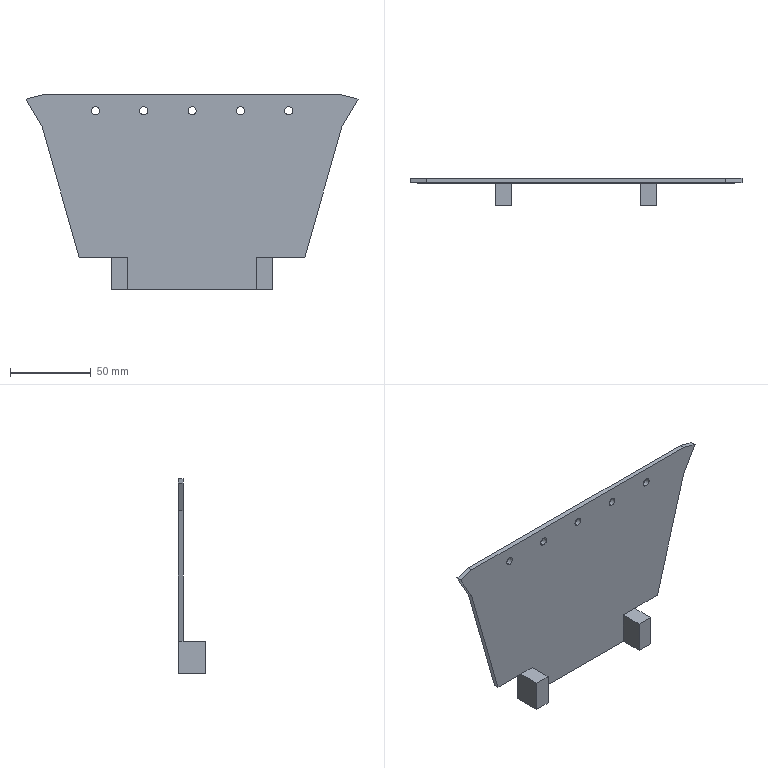Part | STEP file | Bin side panel | 1 solid | 30 faces | box 206.163 x 17 x 120.782 mm | volume 62585 mm3 | plane 20 | cylinder 10 | commonest cylinder face diameters 5.1 x10